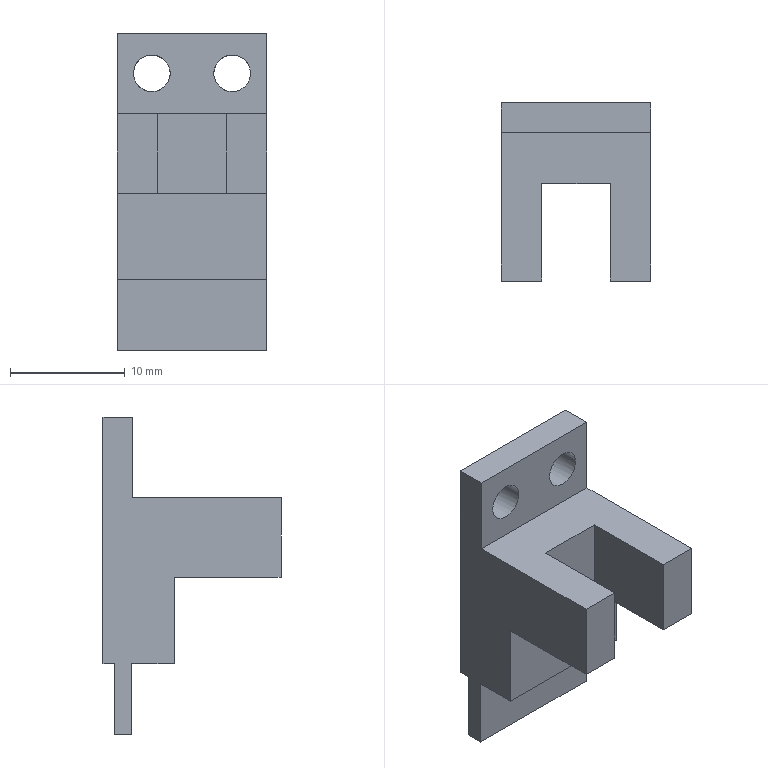Part | NX | 1 solid | 20 faces | box 13 x 15.5 x 27.65 mm | volume 1966 mm3 | plane 18 | cylinder 2 | commonest cylinder face diameters 3.2 x2
STEP:
#1=CARTESIAN_POINT('',(-6.5,-1.,-7.5));
#2=VERTEX_POINT('',#1);
#3=CARTESIAN_POINT('',(6.5,-1.,-7.5));
#4=VERTEX_POINT('',#3);
#5=CARTESIAN_POINT('',(6.5,-1.,-7.5));
#6=DIRECTION('',(1.,0.,0.));
#7=VECTOR('',#6,1000.);
#8=LINE('',#5,#7);
#9=EDGE_CURVE('',#2,#4,#8,.T.);
#10=ORIENTED_EDGE('',*,*,#9,.F.);
#11=CARTESIAN_POINT('',(-6.5,0.,-7.5));
#12=VERTEX_POINT('',#11);
#13=CARTESIAN_POINT('',(-6.5,0.,-7.5));
#14=DIRECTION('',(0.,1.,0.));
#15=VECTOR('',#14,1000.);
#16=LINE('',#13,#15);
#17=EDGE_CURVE('',#2,#12,#16,.T.);
#18=ORIENTED_EDGE('',*,*,#17,.T.);
#19=CARTESIAN_POINT('',(6.5,0.,-7.5));
#20=VERTEX_POINT('',#19);
#21=CARTESIAN_POINT('',(6.5,0.,-7.5));
#22=DIRECTION('',(1.,0.,0.));
#23=VECTOR('',#22,1000.);
#24=LINE('',#21,#23);
#25=EDGE_CURVE('',#12,#20,#24,.T.);
#26=ORIENTED_EDGE('',*,*,#25,.T.);
#27=CARTESIAN_POINT('',(6.5,0.,-7.5));
#28=DIRECTION('',(0.,-1.,0.));
#29=VECTOR('',#28,1000.);
#30=LINE('',#27,#29);
#31=EDGE_CURVE('',#20,#4,#30,.T.);
#32=ORIENTED_EDGE('',*,*,#31,.T.);
#33=EDGE_LOOP('',(#10,#18,#26,#32));
#34=FACE_BOUND('',#33,.T.);
#35=CARTESIAN_POINT('',(0.,0.,-7.5));
#36=DIRECTION('',(0.,0.,-1.));
#37=DIRECTION('',(-1.,0.,0.));
#38=AXIS2_PLACEMENT_3D('',#35,#36,#37);
#39=PLANE('',#38);
#40=ADVANCED_FACE('',(#34),#39,.T.);
#41=CARTESIAN_POINT('',(-6.5,-2.6,6.95));
#42=VERTEX_POINT('',#41);
#43=CARTESIAN_POINT('',(6.5,-2.6,6.95));
#44=VERTEX_POINT('',#43);
#45=CARTESIAN_POINT('',(-6.5,-2.6,6.95));
#46=DIRECTION('',(1.,0.,0.));
#47=VECTOR('',#46,1000.);
#48=LINE('',#45,#47);
#49=EDGE_CURVE('',#42,#44,#48,.T.);
#50=ORIENTED_EDGE('',*,*,#49,.F.);
#51=CARTESIAN_POINT('',(-6.5,-15.5,6.95));
#52=VERTEX_POINT('',#51);
#53=CARTESIAN_POINT('',(-6.5,0.,6.95));
#54=DIRECTION('',(0.,-1.,0.));
#55=VECTOR('',#54,1000.);
#56=LINE('',#53,#55);
#57=EDGE_CURVE('',#42,#52,#56,.T.);
#58=ORIENTED_EDGE('',*,*,#57,.T.);
#59=CARTESIAN_POINT('',(-3.,-15.5,6.95));
#60=VERTEX_POINT('',#59);
#61=CARTESIAN_POINT('',(-6.5,-15.5,6.95));
#62=DIRECTION('',(1.,0.,0.));
#63=VECTOR('',#62,1000.);
#64=LINE('',#61,#63);
#65=EDGE_CURVE('',#52,#60,#64,.T.);
#66=ORIENTED_EDGE('',*,*,#65,.T.);
#67=CARTESIAN_POINT('',(-3.,-7.,6.95));
#68=VERTEX_POINT('',#67);
#69=CARTESIAN_POINT('',(-3.,-15.5,6.95));
#70=DIRECTION('',(0.,1.,0.));
#71=VECTOR('',#70,1000.);
#72=LINE('',#69,#71);
#73=EDGE_CURVE('',#60,#68,#72,.T.);
#74=ORIENTED_EDGE('',*,*,#73,.T.);
#75=CARTESIAN_POINT('',(3.,-7.,6.95));
#76=VERTEX_POINT('',#75);
#77=CARTESIAN_POINT('',(-3.,-7.,6.95));
#78=DIRECTION('',(1.,0.,0.));
#79=VECTOR('',#78,1000.);
#80=LINE('',#77,#79);
#81=EDGE_CURVE('',#68,#76,#80,.T.);
#82=ORIENTED_EDGE('',*,*,#81,.T.);
#83=CARTESIAN_POINT('',(3.,-15.5,6.95));
#84=VERTEX_POINT('',#83);
#85=CARTESIAN_POINT('',(3.,-15.5,6.95));
#86=DIRECTION('',(0.,-1.,0.));
#87=VECTOR('',#86,1000.);
#88=LINE('',#85,#87);
#89=EDGE_CURVE('',#76,#84,#88,.T.);
#90=ORIENTED_EDGE('',*,*,#89,.T.);
#91=CARTESIAN_POINT('',(6.5,-15.5,6.95));
#92=VERTEX_POINT('',#91);
#93=CARTESIAN_POINT('',(6.5,-15.5,6.95));
#94=DIRECTION('',(1.,0.,0.));
#95=VECTOR('',#94,1000.);
#96=LINE('',#93,#95);
#97=EDGE_CURVE('',#84,#92,#96,.T.);
#98=ORIENTED_EDGE('',*,*,#97,.T.);
#99=CARTESIAN_POINT('',(6.5,0.,6.95));
#100=DIRECTION('',(0.,1.,0.));
#101=VECTOR('',#100,1000.);
#102=LINE('',#99,#101);
#103=EDGE_CURVE('',#92,#44,#102,.T.);
#104=ORIENTED_EDGE('',*,*,#103,.T.);
#105=EDGE_LOOP('',(#50,#58,#66,#74,#82,#90,#98,#104));
#106=FACE_BOUND('',#105,.T.);
#107=CARTESIAN_POINT('',(0.,0.,6.95));
#108=DIRECTION('',(0.,0.,-1.));
#109=DIRECTION('',(-1.,0.,0.));
#110=AXIS2_PLACEMENT_3D('',#107,#108,#109);
#111=PLANE('',#110);
#112=ADVANCED_FACE('',(#106),#111,.F.);
#113=CARTESIAN_POINT('',(6.5,-15.5,0.));
#114=VERTEX_POINT('',#113);
#115=CARTESIAN_POINT('',(6.5,-6.2,0.));
#116=VERTEX_POINT('',#115);
#117=CARTESIAN_POINT('',(6.5,0.,0.));
#118=DIRECTION('',(0.,1.,0.));
#119=VECTOR('',#118,1000.);
#120=LINE('',#117,#119);
#121=EDGE_CURVE('',#114,#116,#120,.T.);
#122=ORIENTED_EDGE('',*,*,#121,.T.);
#123=CARTESIAN_POINT('',(6.5,-6.2,-7.5));
#124=VERTEX_POINT('',#123);
#125=CARTESIAN_POINT('',(6.5,-6.2,-7.5));
#126=DIRECTION('',(0.,0.,1.));
#127=VECTOR('',#126,1000.);
#128=LINE('',#125,#127);
#129=EDGE_CURVE('',#124,#116,#128,.T.);
#130=ORIENTED_EDGE('',*,*,#129,.F.);
#131=CARTESIAN_POINT('',(6.5,-2.5,-7.5));
#132=VERTEX_POINT('',#131);
#133=CARTESIAN_POINT('',(6.5,0.,-7.5));
#134=DIRECTION('',(0.,-1.,0.));
#135=VECTOR('',#134,1000.);
#136=LINE('',#133,#135);
#137=EDGE_CURVE('',#132,#124,#136,.T.);
#138=ORIENTED_EDGE('',*,*,#137,.F.);
#139=CARTESIAN_POINT('',(6.5,-2.5,-13.7));
#140=VERTEX_POINT('',#139);
#141=CARTESIAN_POINT('',(6.5,-2.5,-13.7));
#142=DIRECTION('',(0.,0.,1.));
#143=VECTOR('',#142,1000.);
#144=LINE('',#141,#143);
#145=EDGE_CURVE('',#140,#132,#144,.T.);
#146=ORIENTED_EDGE('',*,*,#145,.F.);
#147=CARTESIAN_POINT('',(6.5,-1.,-13.7));
#148=VERTEX_POINT('',#147);
#149=CARTESIAN_POINT('',(6.5,-1.,-13.7));
#150=DIRECTION('',(0.,-1.,0.));
#151=VECTOR('',#150,1000.);
#152=LINE('',#149,#151);
#153=EDGE_CURVE('',#148,#140,#152,.T.);
#154=ORIENTED_EDGE('',*,*,#153,.F.);
#155=CARTESIAN_POINT('',(6.5,-1.,-13.7));
#156=DIRECTION('',(0.,0.,1.));
#157=VECTOR('',#156,1000.);
#158=LINE('',#155,#157);
#159=EDGE_CURVE('',#148,#4,#158,.T.);
#160=ORIENTED_EDGE('',*,*,#159,.T.);
#161=ORIENTED_EDGE('',*,*,#31,.F.);
#162=CARTESIAN_POINT('',(6.5,0.,13.95));
#163=VERTEX_POINT('',#162);
#164=CARTESIAN_POINT('',(6.5,0.,6.95));
#165=DIRECTION('',(0.,0.,-1.));
#166=VECTOR('',#165,1000.);
#167=LINE('',#164,#166);
#168=EDGE_CURVE('',#163,#20,#167,.T.);
#169=ORIENTED_EDGE('',*,*,#168,.F.);
#170=CARTESIAN_POINT('',(6.5,-2.6,13.95));
#171=VERTEX_POINT('',#170);
#172=CARTESIAN_POINT('',(6.5,0.,13.95));
#173=DIRECTION('',(0.,1.,0.));
#174=VECTOR('',#173,1000.);
#175=LINE('',#172,#174);
#176=EDGE_CURVE('',#171,#163,#175,.T.);
#177=ORIENTED_EDGE('',*,*,#176,.F.);
#178=CARTESIAN_POINT('',(6.5,-2.6,13.95));
#179=DIRECTION('',(0.,0.,-1.));
#180=VECTOR('',#179,1000.);
#181=LINE('',#178,#180);
#182=EDGE_CURVE('',#171,#44,#181,.T.);
#183=ORIENTED_EDGE('',*,*,#182,.T.);
#184=ORIENTED_EDGE('',*,*,#103,.F.);
#185=CARTESIAN_POINT('',(6.5,-15.5,6.95));
#186=DIRECTION('',(0.,0.,-1.));
#187=VECTOR('',#186,1000.);
#188=LINE('',#185,#187);
#189=EDGE_CURVE('',#92,#114,#188,.T.);
#190=ORIENTED_EDGE('',*,*,#189,.T.);
#191=EDGE_LOOP('',(#122,#130,#138,#146,#154,#160,#161,#169,#177,#183,#184,#190));
#192=FACE_BOUND('',#191,.T.);
#193=CARTESIAN_POINT('',(6.5,0.,6.95));
#194=DIRECTION('',(-1.,0.,0.));
#195=DIRECTION('',(0.,-1.,0.));
#196=AXIS2_PLACEMENT_3D('',#193,#194,#195);
#197=PLANE('',#196);
#198=ADVANCED_FACE('',(#192),#197,.F.);
#199=CARTESIAN_POINT('',(-1.9,0.,10.45));
#200=VERTEX_POINT('',#199);
#201=CARTESIAN_POINT('',(-3.5,0.,10.45));
#202=DIRECTION('',(0.,-1.,0.));
#203=DIRECTION('',(1.,0.,0.));
#204=AXIS2_PLACEMENT_3D('',#201,#202,#203);
#205=CIRCLE('',#204,1.6);
#206=EDGE_CURVE('',#200,#200,#205,.T.);
#207=ORIENTED_EDGE('',*,*,#206,.T.);
#208=EDGE_LOOP('',(#207));
#209=FACE_BOUND('',#208,.T.);
#210=CARTESIAN_POINT('',(5.1,0.,10.45));
#211=VERTEX_POINT('',#210);
#212=CARTESIAN_POINT('',(3.5,0.,10.45));
#213=DIRECTION('',(0.,-1.,0.));
#214=DIRECTION('',(1.,0.,0.));
#215=AXIS2_PLACEMENT_3D('',#212,#213,#214);
#216=CIRCLE('',#215,1.6);
#217=EDGE_CURVE('',#211,#211,#216,.T.);
#218=ORIENTED_EDGE('',*,*,#217,.T.);
#219=EDGE_LOOP('',(#218));
#220=FACE_BOUND('',#219,.T.);
#221=ORIENTED_EDGE('',*,*,#168,.T.);
#222=ORIENTED_EDGE('',*,*,#25,.F.);
#223=CARTESIAN_POINT('',(-6.5,0.,13.95));
#224=VERTEX_POINT('',#223);
#225=CARTESIAN_POINT('',(-6.5,0.,6.95));
#226=DIRECTION('',(0.,0.,-1.));
#227=VECTOR('',#226,1000.);
#228=LINE('',#225,#227);
#229=EDGE_CURVE('',#224,#12,#228,.T.);
#230=ORIENTED_EDGE('',*,*,#229,.F.);
#231=CARTESIAN_POINT('',(-6.5,0.,13.95));
#232=DIRECTION('',(-1.,0.,0.));
#233=VECTOR('',#232,1000.);
#234=LINE('',#231,#233);
#235=EDGE_CURVE('',#163,#224,#234,.T.);
#236=ORIENTED_EDGE('',*,*,#235,.F.);
#237=EDGE_LOOP('',(#221,#222,#230,#236));
#238=FACE_BOUND('',#237,.T.);
#239=CARTESIAN_POINT('',(-6.5,0.,6.95));
#240=DIRECTION('',(0.,-1.,0.));
#241=DIRECTION('',(1.,0.,0.));
#242=AXIS2_PLACEMENT_3D('',#239,#240,#241);
#243=PLANE('',#242);
#244=ADVANCED_FACE('',(#209,#220,#238),#243,.F.);
#245=ORIENTED_EDGE('',*,*,#229,.T.);
#246=ORIENTED_EDGE('',*,*,#17,.F.);
#247=CARTESIAN_POINT('',(-6.5,-1.,-13.7));
#248=VERTEX_POINT('',#247);
#249=CARTESIAN_POINT('',(-6.5,-1.,-13.7));
#250=DIRECTION('',(0.,0.,1.));
#251=VECTOR('',#250,1000.);
#252=LINE('',#249,#251);
#253=EDGE_CURVE('',#248,#2,#252,.T.);
#254=ORIENTED_EDGE('',*,*,#253,.F.);
#255=CARTESIAN_POINT('',(-6.5,-2.5,-13.7));
#256=VERTEX_POINT('',#255);
#257=CARTESIAN_POINT('',(-6.5,-1.,-13.7));
#258=DIRECTION('',(0.,1.,0.));
#259=VECTOR('',#258,1000.);
#260=LINE('',#257,#259);
#261=EDGE_CURVE('',#256,#248,#260,.T.);
#262=ORIENTED_EDGE('',*,*,#261,.F.);
#263=CARTESIAN_POINT('',(-6.5,-2.5,-7.5));
#264=VERTEX_POINT('',#263);
#265=CARTESIAN_POINT('',(-6.5,-2.5,-13.7));
#266=DIRECTION('',(0.,0.,1.));
#267=VECTOR('',#266,1000.);
#268=LINE('',#265,#267);
#269=EDGE_CURVE('',#256,#264,#268,.T.);
#270=ORIENTED_EDGE('',*,*,#269,.T.);
#271=CARTESIAN_POINT('',(-6.5,-6.2,-7.5));
#272=VERTEX_POINT('',#271);
#273=CARTESIAN_POINT('',(-6.5,0.,-7.5));
#274=DIRECTION('',(0.,1.,0.));
#275=VECTOR('',#274,1000.);
#276=LINE('',#273,#275);
#277=EDGE_CURVE('',#272,#264,#276,.T.);
#278=ORIENTED_EDGE('',*,*,#277,.F.);
#279=CARTESIAN_POINT('',(-6.5,-6.2,0.));
#280=VERTEX_POINT('',#279);
#281=CARTESIAN_POINT('',(-6.5,-6.2,-7.5));
#282=DIRECTION('',(0.,0.,1.));
#283=VECTOR('',#282,1000.);
#284=LINE('',#281,#283);
#285=EDGE_CURVE('',#272,#280,#284,.T.);
#286=ORIENTED_EDGE('',*,*,#285,.T.);
#287=CARTESIAN_POINT('',(-6.5,-15.5,0.));
#288=VERTEX_POINT('',#287);
#289=CARTESIAN_POINT('',(-6.5,0.,0.));
#290=DIRECTION('',(0.,-1.,0.));
#291=VECTOR('',#290,1000.);
#292=LINE('',#289,#291);
#293=EDGE_CURVE('',#280,#288,#292,.T.);
#294=ORIENTED_EDGE('',*,*,#293,.T.);
#295=CARTESIAN_POINT('',(-6.5,-15.5,6.95));
#296=DIRECTION('',(0.,0.,-1.));
#297=VECTOR('',#296,1000.);
#298=LINE('',#295,#297);
#299=EDGE_CURVE('',#52,#288,#298,.T.);
#300=ORIENTED_EDGE('',*,*,#299,.F.);
#301=ORIENTED_EDGE('',*,*,#57,.F.);
#302=CARTESIAN_POINT('',(-6.5,-2.6,13.95));
#303=VERTEX_POINT('',#302);
#304=CARTESIAN_POINT('',(-6.5,-2.6,13.95));
#305=DIRECTION('',(0.,0.,-1.));
#306=VECTOR('',#305,1000.);
#307=LINE('',#304,#306);
#308=EDGE_CURVE('',#303,#42,#307,.T.);
#309=ORIENTED_EDGE('',*,*,#308,.F.);
#310=CARTESIAN_POINT('',(-6.5,0.,13.95));
#311=DIRECTION('',(0.,-1.,0.));
#312=VECTOR('',#311,1000.);
#313=LINE('',#310,#312);
#314=EDGE_CURVE('',#224,#303,#313,.T.);
#315=ORIENTED_EDGE('',*,*,#314,.F.);
#316=EDGE_LOOP('',(#245,#246,#254,#262,#270,#278,#286,#294,#300,#301,#309,#315));
#317=FACE_BOUND('',#316,.T.);
#318=CARTESIAN_POINT('',(-6.5,0.,6.95));
#319=DIRECTION('',(1.,0.,0.));
#320=DIRECTION('',(0.,1.,0.));
#321=AXIS2_PLACEMENT_3D('',#318,#319,#320);
#322=PLANE('',#321);
#323=ADVANCED_FACE('',(#317),#322,.F.);
#324=CARTESIAN_POINT('',(-3.,-15.5,0.));
#325=VERTEX_POINT('',#324);
#326=CARTESIAN_POINT('',(-6.5,-15.5,0.));
#327=DIRECTION('',(1.,0.,0.));
#328=VECTOR('',#327,1000.);
#329=LINE('',#326,#328);
#330=EDGE_CURVE('',#288,#325,#329,.T.);
#331=ORIENTED_EDGE('',*,*,#330,.T.);
#332=CARTESIAN_POINT('',(-3.,-15.5,6.95));
#333=DIRECTION('',(0.,0.,-1.));
#334=VECTOR('',#333,1000.);
#335=LINE('',#332,#334);
#336=EDGE_CURVE('',#60,#325,#335,.T.);
#337=ORIENTED_EDGE('',*,*,#336,.F.);
#338=ORIENTED_EDGE('',*,*,#65,.F.);
#339=ORIENTED_EDGE('',*,*,#299,.T.);
#340=EDGE_LOOP('',(#331,#337,#338,#339));
#341=FACE_BOUND('',#340,.T.);
#342=CARTESIAN_POINT('',(-6.5,-15.5,6.95));
#343=DIRECTION('',(0.,1.,0.));
#344=DIRECTION('',(-1.,0.,0.));
#345=AXIS2_PLACEMENT_3D('',#342,#343,#344);
#346=PLANE('',#345);
#347=ADVANCED_FACE('',(#341),#346,.F.);
#348=CARTESIAN_POINT('',(-3.,-7.,0.));
#349=VERTEX_POINT('',#348);
#350=CARTESIAN_POINT('',(-3.,-15.5,0.));
#351=DIRECTION('',(0.,1.,0.));
#352=VECTOR('',#351,1000.);
#353=LINE('',#350,#352);
#354=EDGE_CURVE('',#325,#349,#353,.T.);
#355=ORIENTED_EDGE('',*,*,#354,.T.);
#356=CARTESIAN_POINT('',(-3.,-7.,6.95));
#357=DIRECTION('',(0.,0.,-1.));
#358=VECTOR('',#357,1000.);
#359=LINE('',#356,#358);
#360=EDGE_CURVE('',#68,#349,#359,.T.);
#361=ORIENTED_EDGE('',*,*,#360,.F.);
#362=ORIENTED_EDGE('',*,*,#73,.F.);
#363=ORIENTED_EDGE('',*,*,#336,.T.);
#364=EDGE_LOOP('',(#355,#361,#362,#363));
#365=FACE_BOUND('',#364,.T.);
#366=CARTESIAN_POINT('',(-3.,-15.5,6.95));
#367=DIRECTION('',(-1.,0.,0.));
#368=DIRECTION('',(0.,-1.,0.));
#369=AXIS2_PLACEMENT_3D('',#366,#367,#368);
#370=PLANE('',#369);
#371=ADVANCED_FACE('',(#365),#370,.F.);
#372=CARTESIAN_POINT('',(3.,-7.,0.));
#373=VERTEX_POINT('',#372);
#374=CARTESIAN_POINT('',(-3.,-7.,0.));
#375=DIRECTION('',(1.,0.,0.));
#376=VECTOR('',#375,1000.);
#377=LINE('',#374,#376);
#378=EDGE_CURVE('',#349,#373,#377,.T.);
#379=ORIENTED_EDGE('',*,*,#378,.T.);
#380=CARTESIAN_POINT('',(3.,-7.,6.95));
#381=DIRECTION('',(0.,0.,-1.));
#382=VECTOR('',#381,1000.);
#383=LINE('',#380,#382);
#384=EDGE_CURVE('',#76,#373,#383,.T.);
#385=ORIENTED_EDGE('',*,*,#384,.F.);
#386=ORIENTED_EDGE('',*,*,#81,.F.);
#387=ORIENTED_EDGE('',*,*,#360,.T.);
#388=EDGE_LOOP('',(#379,#385,#386,#387));
#389=FACE_BOUND('',#388,.T.);
#390=CARTESIAN_POINT('',(-3.,-7.,6.95));
#391=DIRECTION('',(0.,1.,0.));
#392=DIRECTION('',(-1.,0.,0.));
#393=AXIS2_PLACEMENT_3D('',#390,#391,#392);
#394=PLANE('',#393);
#395=ADVANCED_FACE('',(#389),#394,.F.);
#396=CARTESIAN_POINT('',(3.,-15.5,0.));
#397=VERTEX_POINT('',#396);
#398=CARTESIAN_POINT('',(3.,-15.5,0.));
#399=DIRECTION('',(0.,-1.,0.));
#400=VECTOR('',#399,1000.);
#401=LINE('',#398,#400);
#402=EDGE_CURVE('',#373,#397,#401,.T.);
#403=ORIENTED_EDGE('',*,*,#402,.T.);
#404=CARTESIAN_POINT('',(3.,-15.5,6.95));
#405=DIRECTION('',(0.,0.,-1.));
#406=VECTOR('',#405,1000.);
#407=LINE('',#404,#406);
#408=EDGE_CURVE('',#84,#397,#407,.T.);
#409=ORIENTED_EDGE('',*,*,#408,.F.);
#410=ORIENTED_EDGE('',*,*,#89,.F.);
#411=ORIENTED_EDGE('',*,*,#384,.T.);
#412=EDGE_LOOP('',(#403,#409,#410,#411));
#413=FACE_BOUND('',#412,.T.);
#414=CARTESIAN_POINT('',(3.,-15.5,6.95));
#415=DIRECTION('',(1.,0.,0.));
#416=DIRECTION('',(0.,1.,0.));
#417=AXIS2_PLACEMENT_3D('',#414,#415,#416);
#418=PLANE('',#417);
#419=ADVANCED_FACE('',(#413),#418,.F.);
#420=CARTESIAN_POINT('',(6.5,-15.5,0.));
#421=DIRECTION('',(1.,0.,0.));
#422=VECTOR('',#421,1000.);
#423=LINE('',#420,#422);
#424=EDGE_CURVE('',#397,#114,#423,.T.);
#425=ORIENTED_EDGE('',*,*,#424,.T.);
#426=ORIENTED_EDGE('',*,*,#189,.F.);
#427=ORIENTED_EDGE('',*,*,#97,.F.);
#428=ORIENTED_EDGE('',*,*,#408,.T.);
#429=EDGE_LOOP('',(#425,#426,#427,#428));
#430=FACE_BOUND('',#429,.T.);
#431=CARTESIAN_POINT('',(6.5,-15.5,6.95));
#432=DIRECTION('',(0.,1.,0.));
#433=DIRECTION('',(0.,0.,1.));
#434=AXIS2_PLACEMENT_3D('',#431,#432,#433);
#435=PLANE('',#434);
#436=ADVANCED_FACE('',(#430),#435,.F.);
#437=CARTESIAN_POINT('',(6.5,-6.2,0.));
#438=DIRECTION('',(-1.,0.,0.));
#439=VECTOR('',#438,1000.);
#440=LINE('',#437,#439);
#441=EDGE_CURVE('',#116,#280,#440,.T.);
#442=ORIENTED_EDGE('',*,*,#441,.F.);
#443=ORIENTED_EDGE('',*,*,#121,.F.);
#444=ORIENTED_EDGE('',*,*,#424,.F.);
#445=ORIENTED_EDGE('',*,*,#402,.F.);
#446=ORIENTED_EDGE('',*,*,#378,.F.);
#447=ORIENTED_EDGE('',*,*,#354,.F.);
#448=ORIENTED_EDGE('',*,*,#330,.F.);
#449=ORIENTED_EDGE('',*,*,#293,.F.);
#450=EDGE_LOOP('',(#442,#443,#444,#445,#446,#447,#448,#449));
#451=FACE_BOUND('',#450,.T.);
#452=CARTESIAN_POINT('',(0.,0.,0.));
#453=DIRECTION('',(0.,0.,-1.));
#454=DIRECTION('',(-1.,0.,0.));
#455=AXIS2_PLACEMENT_3D('',#452,#453,#454);
#456=PLANE('',#455);
#457=ADVANCED_FACE('',(#451),#456,.T.);
#458=CARTESIAN_POINT('',(-3.5,-2.6,8.85));
#459=VERTEX_POINT('',#458);
#460=CARTESIAN_POINT('',(-3.5,-2.6,10.45));
#461=DIRECTION('',(0.,-1.,0.));
#462=DIRECTION('',(0.,0.,-1.));
#463=AXIS2_PLACEMENT_3D('',#460,#461,#462);
#464=CIRCLE('',#463,1.6);
#465=EDGE_CURVE('',#459,#459,#464,.T.);
#466=ORIENTED_EDGE('',*,*,#465,.F.);
#467=EDGE_LOOP('',(#466));
#468=FACE_BOUND('',#467,.T.);
#469=CARTESIAN_POINT('',(3.5,-2.6,8.85));
#470=VERTEX_POINT('',#469);
#471=CARTESIAN_POINT('',(3.5,-2.6,10.45));
#472=DIRECTION('',(0.,-1.,0.));
#473=DIRECTION('',(0.,0.,-1.));
#474=AXIS2_PLACEMENT_3D('',#471,#472,#473);
#475=CIRCLE('',#474,1.6);
#476=EDGE_CURVE('',#470,#470,#475,.T.);
#477=ORIENTED_EDGE('',*,*,#476,.F.);
#478=EDGE_LOOP('',(#477));
#479=FACE_BOUND('',#478,.T.);
#480=ORIENTED_EDGE('',*,*,#49,.T.);
#481=ORIENTED_EDGE('',*,*,#182,.F.);
#482=CARTESIAN_POINT('',(-6.5,-2.6,13.95));
#483=DIRECTION('',(1.,0.,0.));
#484=VECTOR('',#483,1000.);
#485=LINE('',#482,#484);
#486=EDGE_CURVE('',#303,#171,#485,.T.);
#487=ORIENTED_EDGE('',*,*,#486,.F.);
#488=ORIENTED_EDGE('',*,*,#308,.T.);
#489=EDGE_LOOP('',(#480,#481,#487,#488));
#490=FACE_BOUND('',#489,.T.);
#491=CARTESIAN_POINT('',(-6.5,-2.6,13.95));
#492=DIRECTION('',(0.,1.,0.));
#493=DIRECTION('',(0.,0.,1.));
#494=AXIS2_PLACEMENT_3D('',#491,#492,#493);
#495=PLANE('',#494);
#496=ADVANCED_FACE('',(#468,#479,#490),#495,.F.);
#497=ORIENTED_EDGE('',*,*,#314,.T.);
#498=ORIENTED_EDGE('',*,*,#486,.T.);
#499=ORIENTED_EDGE('',*,*,#176,.T.);
#500=ORIENTED_EDGE('',*,*,#235,.T.);
#501=EDGE_LOOP('',(#497,#498,#499,#500));
#502=FACE_BOUND('',#501,.T.);
#503=CARTESIAN_POINT('',(0.,0.,13.95));
#504=DIRECTION('',(0.,0.,1.));
#505=DIRECTION('',(1.,0.,0.));
#506=AXIS2_PLACEMENT_3D('',#503,#504,#505);
#507=PLANE('',#506);
#508=ADVANCED_FACE('',(#502),#507,.T.);
#509=ORIENTED_EDGE('',*,*,#441,.T.);
#510=ORIENTED_EDGE('',*,*,#285,.F.);
#511=CARTESIAN_POINT('',(6.5,-6.2,-7.5));
#512=DIRECTION('',(-1.,0.,0.));
#513=VECTOR('',#512,1000.);
#514=LINE('',#511,#513);
#515=EDGE_CURVE('',#124,#272,#514,.T.);
#516=ORIENTED_EDGE('',*,*,#515,.F.);
#517=ORIENTED_EDGE('',*,*,#129,.T.);
#518=EDGE_LOOP('',(#509,#510,#516,#517));
#519=FACE_BOUND('',#518,.T.);
#520=CARTESIAN_POINT('',(6.5,-6.2,-7.5));
#521=DIRECTION('',(0.,1.,0.));
#522=DIRECTION('',(0.,0.,1.));
#523=AXIS2_PLACEMENT_3D('',#520,#521,#522);
#524=PLANE('',#523);
#525=ADVANCED_FACE('',(#519),#524,.F.);
#526=CARTESIAN_POINT('',(6.5,-2.5,-7.5));
#527=DIRECTION('',(-1.,0.,0.));
#528=VECTOR('',#527,1000.);
#529=LINE('',#526,#528);
#530=EDGE_CURVE('',#132,#264,#529,.T.);
#531=ORIENTED_EDGE('',*,*,#530,.F.);
#532=ORIENTED_EDGE('',*,*,#137,.T.);
#533=ORIENTED_EDGE('',*,*,#515,.T.);
#534=ORIENTED_EDGE('',*,*,#277,.T.);
#535=EDGE_LOOP('',(#531,#532,#533,#534));
#536=FACE_BOUND('',#535,.T.);
#537=CARTESIAN_POINT('',(0.,0.,-7.5));
#538=DIRECTION('',(0.,0.,-1.));
#539=DIRECTION('',(-1.,0.,0.));
#540=AXIS2_PLACEMENT_3D('',#537,#538,#539);
#541=PLANE('',#540);
#542=ADVANCED_FACE('',(#536),#541,.T.);
#543=ORIENTED_EDGE('',*,*,#530,.T.);
#544=ORIENTED_EDGE('',*,*,#269,.F.);
#545=CARTESIAN_POINT('',(6.5,-2.5,-13.7));
#546=DIRECTION('',(-1.,0.,0.));
#547=VECTOR('',#546,1000.);
#548=LINE('',#545,#547);
#549=EDGE_CURVE('',#140,#256,#548,.T.);
#550=ORIENTED_EDGE('',*,*,#549,.F.);
#551=ORIENTED_EDGE('',*,*,#145,.T.);
#552=EDGE_LOOP('',(#543,#544,#550,#551));
#553=FACE_BOUND('',#552,.T.);
#554=CARTESIAN_POINT('',(6.5,-2.5,-13.7));
#555=DIRECTION('',(0.,1.,0.));
#556=DIRECTION('',(0.,0.,1.));
#557=AXIS2_PLACEMENT_3D('',#554,#555,#556);
#558=PLANE('',#557);
#559=ADVANCED_FACE('',(#553),#558,.F.);
#560=ORIENTED_EDGE('',*,*,#9,.T.);
#561=ORIENTED_EDGE('',*,*,#159,.F.);
#562=CARTESIAN_POINT('',(6.5,-1.,-13.7));
#563=DIRECTION('',(1.,0.,0.));
#564=VECTOR('',#563,1000.);
#565=LINE('',#562,#564);
#566=EDGE_CURVE('',#248,#148,#565,.T.);
#567=ORIENTED_EDGE('',*,*,#566,.F.);
#568=ORIENTED_EDGE('',*,*,#253,.T.);
#569=EDGE_LOOP('',(#560,#561,#567,#568));
#570=FACE_BOUND('',#569,.T.);
#571=CARTESIAN_POINT('',(6.5,-1.,-13.7));
#572=DIRECTION('',(0.,-1.,0.));
#573=DIRECTION('',(0.,0.,-1.));
#574=AXIS2_PLACEMENT_3D('',#571,#572,#573);
#575=PLANE('',#574);
#576=ADVANCED_FACE('',(#570),#575,.F.);
#577=ORIENTED_EDGE('',*,*,#153,.T.);
#578=ORIENTED_EDGE('',*,*,#549,.T.);
#579=ORIENTED_EDGE('',*,*,#261,.T.);
#580=ORIENTED_EDGE('',*,*,#566,.T.);
#581=EDGE_LOOP('',(#577,#578,#579,#580));
#582=FACE_BOUND('',#581,.T.);
#583=CARTESIAN_POINT('',(0.,0.,-13.7));
#584=DIRECTION('',(0.,0.,-1.));
#585=DIRECTION('',(-1.,0.,0.));
#586=AXIS2_PLACEMENT_3D('',#583,#584,#585);
#587=PLANE('',#586);
#588=ADVANCED_FACE('',(#582),#587,.T.);
#589=ORIENTED_EDGE('',*,*,#476,.T.);
#590=EDGE_LOOP('',(#589));
#591=FACE_BOUND('',#590,.T.);
#592=ORIENTED_EDGE('',*,*,#217,.F.);
#593=EDGE_LOOP('',(#592));
#594=FACE_BOUND('',#593,.T.);
#595=CARTESIAN_POINT('',(3.5,-2.6,10.45));
#596=DIRECTION('',(0.,-1.,0.));
#597=DIRECTION('',(0.,0.,-1.));
#598=AXIS2_PLACEMENT_3D('',#595,#596,#597);
#599=CYLINDRICAL_SURFACE('',#598,1.6);
#600=ADVANCED_FACE('',(#591,#594),#599,.F.);
#601=ORIENTED_EDGE('',*,*,#465,.T.);
#602=EDGE_LOOP('',(#601));
#603=FACE_BOUND('',#602,.T.);
#604=ORIENTED_EDGE('',*,*,#206,.F.);
#605=EDGE_LOOP('',(#604));
#606=FACE_BOUND('',#605,.T.);
#607=CARTESIAN_POINT('',(-3.5,-2.6,10.45));
#608=DIRECTION('',(0.,-1.,0.));
#609=DIRECTION('',(0.,0.,-1.));
#610=AXIS2_PLACEMENT_3D('',#607,#608,#609);
#611=CYLINDRICAL_SURFACE('',#610,1.6);
#612=ADVANCED_FACE('',(#603,#606),#611,.F.);
#613=CLOSED_SHELL('',(#40,#112,#198,#244,#323,#347,#371,#395,#419,#436,#457,#496,#508,#525,#542,#559,#576,#588,#600,#612));
#614=MANIFOLD_SOLID_BREP('',#613);
#615=(LENGTH_UNIT()NAMED_UNIT(*)SI_UNIT(.MILLI.,.METRE.));
#616=UNCERTAINTY_MEASURE_WITH_UNIT(LENGTH_MEASURE(0.00001),#615,'','');
#617=(NAMED_UNIT(*)PLANE_ANGLE_UNIT()SI_UNIT($,.RADIAN.));
#618=(NAMED_UNIT(*)SI_UNIT($,.STERADIAN.)SOLID_ANGLE_UNIT());
#619=(GEOMETRIC_REPRESENTATION_CONTEXT(3)GLOBAL_UNCERTAINTY_ASSIGNED_CONTEXT((#616))GLOBAL_UNIT_ASSIGNED_CONTEXT((#615,#617,#618))REPRESENTATION_CONTEXT('',''));
#620=ADVANCED_BREP_SHAPE_REPRESENTATION('',(#614),#619);